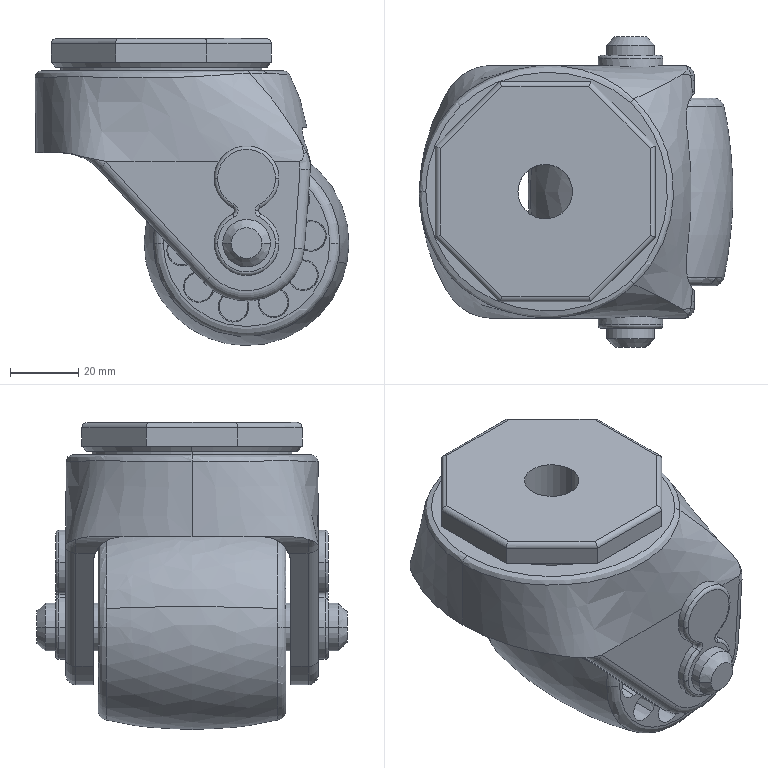Part | STEP file | ~ACM-600S.stp | 1 solid | 199 faces | box 91.981 x 91 x 90 mm | volume 300856 mm3 | cylinder 55 | plane 51 | cone 50 | torus 26 | spline 17 | commonest cylinder face diameters 19 x12 3 x8 14 x8 2 x6 6 x4 16 x4